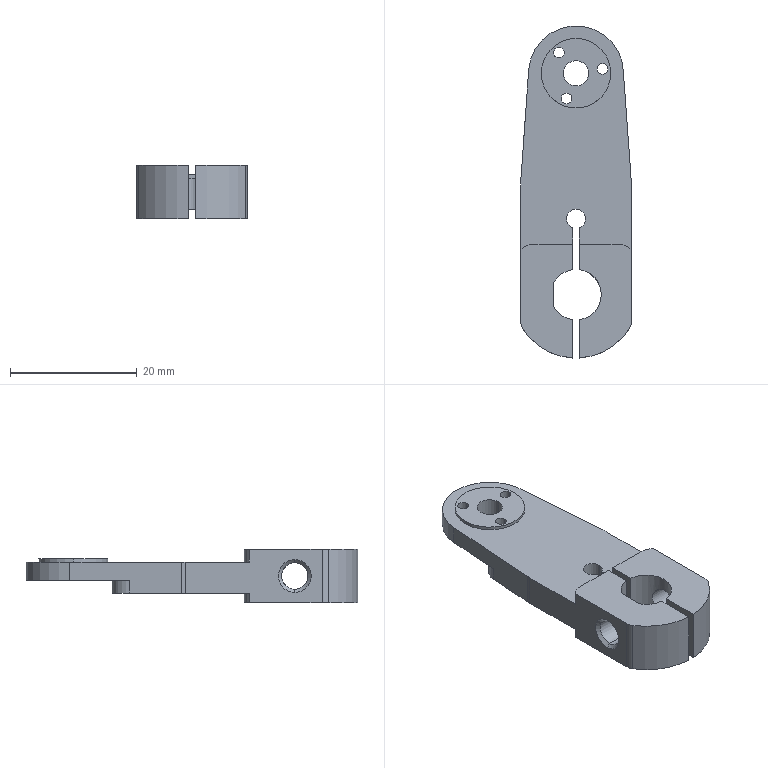Part | NX | features BREP 1 | 1 solid | 61 faces | box 17.477 x 52.487 x 8.4 mm | volume 3967 mm3 | cylinder 35 | plane 22 | cone 4 | commonest cylinder face diameters 1.7 x6 6 x6 4 x4 4.2 x4 3 x3 8 x3